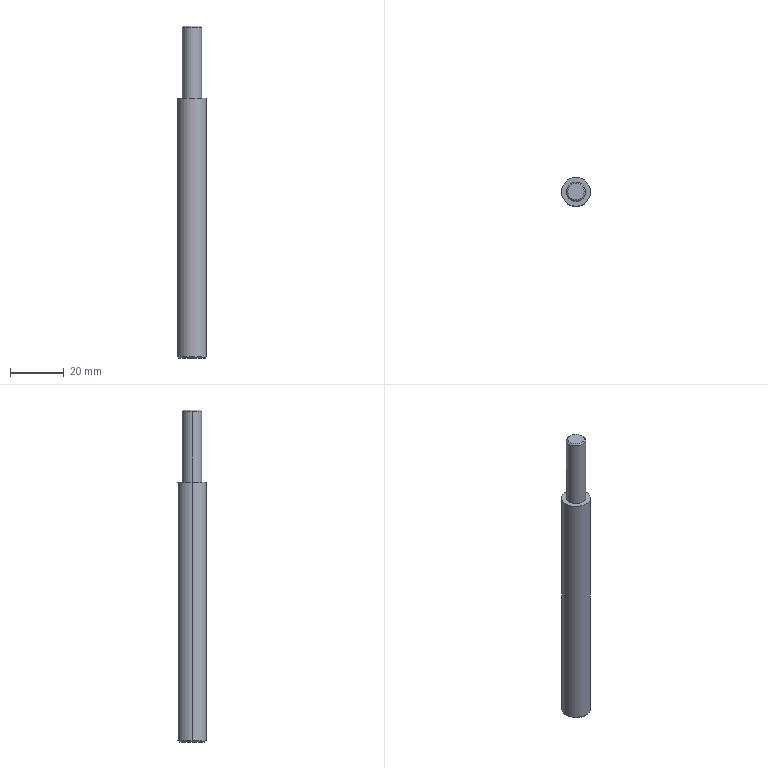Part | SolidWorks | features Chamfer 1, Extrusion 1, ICE 1 | 1 solid | 11 faces | box 10.8 x 10.8 x 124 mm | volume 9977 mm3 | cone 4 | cylinder 4 | plane 3 | commonest cylinder face diameters 7.2 x2 10.8 x2
STEP:
#1=CARTESIAN_POINT('',(3.06,0.,124.));
#2=VERTEX_POINT('',#1);
#3=CARTESIAN_POINT('',(-3.06,0.,124.));
#4=VERTEX_POINT('',#3);
#5=CARTESIAN_POINT('',(0.,0.,124.));
#6=DIRECTION('',(0.,0.,1.));
#7=DIRECTION('',(1.,0.,0.));
#8=AXIS2_PLACEMENT_3D('',#5,#6,#7);
#9=CIRCLE('',#8,3.06);
#10=EDGE_CURVE('',#2,#4,#9,.T.);
#11=ORIENTED_EDGE('',*,*,#10,.F.);
#12=CARTESIAN_POINT('',(3.6,0.,123.46));
#13=VERTEX_POINT('',#12);
#14=CARTESIAN_POINT('',(3.06,0.,124.));
#15=DIRECTION('',(0.7071,0.,-0.7071));
#16=VECTOR('',#15,1000.);
#17=LINE('',#14,#16);
#18=EDGE_CURVE('',#2,#13,#17,.T.);
#19=ORIENTED_EDGE('',*,*,#18,.T.);
#20=CARTESIAN_POINT('',(-3.6,0.,123.46));
#21=VERTEX_POINT('',#20);
#22=CARTESIAN_POINT('',(0.,0.,123.46));
#23=DIRECTION('',(0.,0.,-1.));
#24=DIRECTION('',(1.,0.,0.));
#25=AXIS2_PLACEMENT_3D('',#22,#23,#24);
#26=CIRCLE('',#25,3.6);
#27=EDGE_CURVE('',#21,#13,#26,.T.);
#28=ORIENTED_EDGE('',*,*,#27,.F.);
#29=CARTESIAN_POINT('',(-3.06,0.,124.));
#30=DIRECTION('',(-0.7071,0.,-0.7071));
#31=VECTOR('',#30,1000.);
#32=LINE('',#29,#31);
#33=EDGE_CURVE('',#4,#21,#32,.T.);
#34=ORIENTED_EDGE('',*,*,#33,.F.);
#35=EDGE_LOOP('',(#11,#19,#28,#34));
#36=FACE_OUTER_BOUND('',#35,.T.);
#37=CARTESIAN_POINT('',(0.,0.,124.));
#38=DIRECTION('',(0.,0.,-1.));
#39=DIRECTION('',(-1.,0.,0.));
#40=AXIS2_PLACEMENT_3D('',#37,#38,#39);
#41=CONICAL_SURFACE('',#40,3.06,0.7854);
#42=ADVANCED_FACE('',(#36),#41,.T.);
#43=CARTESIAN_POINT('',(-4.86,0.,0.));
#44=VERTEX_POINT('',#43);
#45=CARTESIAN_POINT('',(4.86,0.,0.));
#46=VERTEX_POINT('',#45);
#47=CARTESIAN_POINT('',(0.,0.,0.));
#48=DIRECTION('',(0.,0.,-1.));
#49=DIRECTION('',(1.,0.,0.));
#50=AXIS2_PLACEMENT_3D('',#47,#48,#49);
#51=CIRCLE('',#50,4.86);
#52=EDGE_CURVE('',#44,#46,#51,.T.);
#53=ORIENTED_EDGE('',*,*,#52,.F.);
#54=CARTESIAN_POINT('',(-5.4,0.,0.54));
#55=VERTEX_POINT('',#54);
#56=CARTESIAN_POINT('',(-5.4,0.,0.54));
#57=DIRECTION('',(-0.7071,0.,0.7071));
#58=VECTOR('',#57,1000.);
#59=LINE('',#56,#58);
#60=EDGE_CURVE('',#44,#55,#59,.T.);
#61=ORIENTED_EDGE('',*,*,#60,.T.);
#62=CARTESIAN_POINT('',(5.4,0.,0.54));
#63=VERTEX_POINT('',#62);
#64=CARTESIAN_POINT('',(0.,0.,0.54));
#65=DIRECTION('',(0.,0.,1.));
#66=DIRECTION('',(1.,0.,0.));
#67=AXIS2_PLACEMENT_3D('',#64,#65,#66);
#68=CIRCLE('',#67,5.4);
#69=EDGE_CURVE('',#63,#55,#68,.T.);
#70=ORIENTED_EDGE('',*,*,#69,.F.);
#71=CARTESIAN_POINT('',(5.4,0.,0.54));
#72=DIRECTION('',(0.7071,0.,0.7071));
#73=VECTOR('',#72,1000.);
#74=LINE('',#71,#73);
#75=EDGE_CURVE('',#46,#63,#74,.T.);
#76=ORIENTED_EDGE('',*,*,#75,.F.);
#77=EDGE_LOOP('',(#53,#61,#70,#76));
#78=FACE_OUTER_BOUND('',#77,.T.);
#79=CARTESIAN_POINT('',(0.,0.,0.54));
#80=DIRECTION('',(0.,0.,1.));
#81=DIRECTION('',(1.,0.,0.));
#82=AXIS2_PLACEMENT_3D('',#79,#80,#81);
#83=CONICAL_SURFACE('',#82,5.4,0.7854);
#84=ADVANCED_FACE('',(#78),#83,.T.);
#85=CARTESIAN_POINT('',(3.6,0.,97.));
#86=VERTEX_POINT('',#85);
#87=CARTESIAN_POINT('',(-3.6,0.,97.));
#88=VERTEX_POINT('',#87);
#89=CARTESIAN_POINT('',(0.,0.,97.));
#90=DIRECTION('',(0.,0.,1.));
#91=DIRECTION('',(1.,0.,0.));
#92=AXIS2_PLACEMENT_3D('',#89,#90,#91);
#93=CIRCLE('',#92,3.6);
#94=EDGE_CURVE('',#86,#88,#93,.T.);
#95=ORIENTED_EDGE('',*,*,#94,.T.);
#96=CARTESIAN_POINT('',(-3.6,0.,97.));
#97=DIRECTION('',(0.,0.,1.));
#98=VECTOR('',#97,1000.);
#99=LINE('',#96,#98);
#100=EDGE_CURVE('',#88,#21,#99,.T.);
#101=ORIENTED_EDGE('',*,*,#100,.T.);
#102=ORIENTED_EDGE('',*,*,#27,.T.);
#103=CARTESIAN_POINT('',(3.6,0.,97.));
#104=DIRECTION('',(0.,0.,1.));
#105=VECTOR('',#104,1000.);
#106=LINE('',#103,#105);
#107=EDGE_CURVE('',#86,#13,#106,.T.);
#108=ORIENTED_EDGE('',*,*,#107,.F.);
#109=EDGE_LOOP('',(#95,#101,#102,#108));
#110=FACE_OUTER_BOUND('',#109,.T.);
#111=CARTESIAN_POINT('',(0.,0.,97.));
#112=DIRECTION('',(0.,0.,1.));
#113=DIRECTION('',(1.,0.,0.));
#114=AXIS2_PLACEMENT_3D('',#111,#112,#113);
#115=CYLINDRICAL_SURFACE('',#114,3.6);
#116=ADVANCED_FACE('',(#110),#115,.T.);
#117=CARTESIAN_POINT('',(5.4,0.,97.));
#118=VERTEX_POINT('',#117);
#119=CARTESIAN_POINT('',(-5.4,0.,97.));
#120=VERTEX_POINT('',#119);
#121=CARTESIAN_POINT('',(0.,0.,97.));
#122=DIRECTION('',(0.,0.,1.));
#123=DIRECTION('',(1.,0.,0.));
#124=AXIS2_PLACEMENT_3D('',#121,#122,#123);
#125=CIRCLE('',#124,5.4);
#126=EDGE_CURVE('',#118,#120,#125,.T.);
#127=ORIENTED_EDGE('',*,*,#126,.F.);
#128=CARTESIAN_POINT('',(5.4,0.,124.));
#129=DIRECTION('',(0.,0.,-1.));
#130=VECTOR('',#129,1000.);
#131=LINE('',#128,#130);
#132=EDGE_CURVE('',#118,#63,#131,.T.);
#133=ORIENTED_EDGE('',*,*,#132,.T.);
#134=ORIENTED_EDGE('',*,*,#69,.T.);
#135=CARTESIAN_POINT('',(-5.4,0.,124.));
#136=DIRECTION('',(0.,0.,-1.));
#137=VECTOR('',#136,1000.);
#138=LINE('',#135,#137);
#139=EDGE_CURVE('',#120,#55,#138,.T.);
#140=ORIENTED_EDGE('',*,*,#139,.F.);
#141=EDGE_LOOP('',(#127,#133,#134,#140));
#142=FACE_OUTER_BOUND('',#141,.T.);
#143=CARTESIAN_POINT('',(0.,0.,124.));
#144=DIRECTION('',(0.,0.,-1.));
#145=DIRECTION('',(-1.,0.,0.));
#146=AXIS2_PLACEMENT_3D('',#143,#144,#145);
#147=CYLINDRICAL_SURFACE('',#146,5.4);
#148=ADVANCED_FACE('',(#142),#147,.T.);
#149=ORIENTED_EDGE('',*,*,#132,.F.);
#150=CARTESIAN_POINT('',(0.,0.,97.));
#151=DIRECTION('',(0.,0.,1.));
#152=DIRECTION('',(1.,0.,0.));
#153=AXIS2_PLACEMENT_3D('',#150,#151,#152);
#154=CIRCLE('',#153,5.4);
#155=EDGE_CURVE('',#120,#118,#154,.T.);
#156=ORIENTED_EDGE('',*,*,#155,.F.);
#157=ORIENTED_EDGE('',*,*,#139,.T.);
#158=CARTESIAN_POINT('',(0.,0.,0.54));
#159=DIRECTION('',(0.,0.,1.));
#160=DIRECTION('',(1.,0.,0.));
#161=AXIS2_PLACEMENT_3D('',#158,#159,#160);
#162=CIRCLE('',#161,5.4);
#163=EDGE_CURVE('',#55,#63,#162,.T.);
#164=ORIENTED_EDGE('',*,*,#163,.T.);
#165=EDGE_LOOP('',(#149,#156,#157,#164));
#166=FACE_OUTER_BOUND('',#165,.T.);
#167=CARTESIAN_POINT('',(0.,0.,124.));
#168=DIRECTION('',(0.,0.,-1.));
#169=DIRECTION('',(-1.,0.,0.));
#170=AXIS2_PLACEMENT_3D('',#167,#168,#169);
#171=CYLINDRICAL_SURFACE('',#170,5.4);
#172=ADVANCED_FACE('',(#166),#171,.T.);
#173=CARTESIAN_POINT('',(0.,0.,0.));
#174=DIRECTION('',(0.,0.,-1.));
#175=DIRECTION('',(1.,0.,0.));
#176=AXIS2_PLACEMENT_3D('',#173,#174,#175);
#177=CIRCLE('',#176,4.86);
#178=EDGE_CURVE('',#46,#44,#177,.T.);
#179=ORIENTED_EDGE('',*,*,#178,.T.);
#180=ORIENTED_EDGE('',*,*,#52,.T.);
#181=EDGE_LOOP('',(#179,#180));
#182=FACE_OUTER_BOUND('',#181,.T.);
#183=CARTESIAN_POINT('',(0.,0.,0.));
#184=DIRECTION('',(0.,0.,1.));
#185=DIRECTION('',(1.,0.,0.));
#186=AXIS2_PLACEMENT_3D('',#183,#184,#185);
#187=PLANE('',#186);
#188=ADVANCED_FACE('',(#182),#187,.F.);
#189=ORIENTED_EDGE('',*,*,#94,.F.);
#190=CARTESIAN_POINT('',(0.,0.,97.));
#191=DIRECTION('',(0.,0.,1.));
#192=DIRECTION('',(1.,0.,0.));
#193=AXIS2_PLACEMENT_3D('',#190,#191,#192);
#194=CIRCLE('',#193,3.6);
#195=EDGE_CURVE('',#88,#86,#194,.T.);
#196=ORIENTED_EDGE('',*,*,#195,.F.);
#197=EDGE_LOOP('',(#189,#196));
#198=FACE_BOUND('',#197,.T.);
#199=ORIENTED_EDGE('',*,*,#155,.T.);
#200=ORIENTED_EDGE('',*,*,#126,.T.);
#201=EDGE_LOOP('',(#199,#200));
#202=FACE_OUTER_BOUND('',#201,.T.);
#203=CARTESIAN_POINT('',(0.,0.,97.));
#204=DIRECTION('',(0.,0.,1.));
#205=DIRECTION('',(1.,0.,0.));
#206=AXIS2_PLACEMENT_3D('',#203,#204,#205);
#207=PLANE('',#206);
#208=ADVANCED_FACE('',(#198,#202),#207,.T.);
#209=ORIENTED_EDGE('',*,*,#100,.F.);
#210=ORIENTED_EDGE('',*,*,#195,.T.);
#211=ORIENTED_EDGE('',*,*,#107,.T.);
#212=CARTESIAN_POINT('',(0.,0.,123.46));
#213=DIRECTION('',(0.,0.,-1.));
#214=DIRECTION('',(1.,0.,0.));
#215=AXIS2_PLACEMENT_3D('',#212,#213,#214);
#216=CIRCLE('',#215,3.6);
#217=EDGE_CURVE('',#13,#21,#216,.T.);
#218=ORIENTED_EDGE('',*,*,#217,.T.);
#219=EDGE_LOOP('',(#209,#210,#211,#218));
#220=FACE_OUTER_BOUND('',#219,.T.);
#221=CARTESIAN_POINT('',(0.,0.,97.));
#222=DIRECTION('',(0.,0.,1.));
#223=DIRECTION('',(1.,0.,0.));
#224=AXIS2_PLACEMENT_3D('',#221,#222,#223);
#225=CYLINDRICAL_SURFACE('',#224,3.6);
#226=ADVANCED_FACE('',(#220),#225,.T.);
#227=CARTESIAN_POINT('',(0.,0.,124.));
#228=DIRECTION('',(0.,0.,1.));
#229=DIRECTION('',(1.,0.,0.));
#230=AXIS2_PLACEMENT_3D('',#227,#228,#229);
#231=CIRCLE('',#230,3.06);
#232=EDGE_CURVE('',#4,#2,#231,.T.);
#233=ORIENTED_EDGE('',*,*,#232,.T.);
#234=ORIENTED_EDGE('',*,*,#10,.T.);
#235=EDGE_LOOP('',(#233,#234));
#236=FACE_OUTER_BOUND('',#235,.T.);
#237=CARTESIAN_POINT('',(0.,0.,124.));
#238=DIRECTION('',(0.,0.,1.));
#239=DIRECTION('',(1.,0.,0.));
#240=AXIS2_PLACEMENT_3D('',#237,#238,#239);
#241=PLANE('',#240);
#242=ADVANCED_FACE('',(#236),#241,.T.);
#243=ORIENTED_EDGE('',*,*,#60,.F.);
#244=ORIENTED_EDGE('',*,*,#178,.F.);
#245=ORIENTED_EDGE('',*,*,#75,.T.);
#246=ORIENTED_EDGE('',*,*,#163,.F.);
#247=EDGE_LOOP('',(#243,#244,#245,#246));
#248=FACE_OUTER_BOUND('',#247,.T.);
#249=CARTESIAN_POINT('',(0.,0.,0.54));
#250=DIRECTION('',(0.,0.,1.));
#251=DIRECTION('',(1.,0.,0.));
#252=AXIS2_PLACEMENT_3D('',#249,#250,#251);
#253=CONICAL_SURFACE('',#252,5.4,0.7854);
#254=ADVANCED_FACE('',(#248),#253,.T.);
#255=ORIENTED_EDGE('',*,*,#18,.F.);
#256=ORIENTED_EDGE('',*,*,#232,.F.);
#257=ORIENTED_EDGE('',*,*,#33,.T.);
#258=ORIENTED_EDGE('',*,*,#217,.F.);
#259=EDGE_LOOP('',(#255,#256,#257,#258));
#260=FACE_OUTER_BOUND('',#259,.T.);
#261=CARTESIAN_POINT('',(0.,0.,124.));
#262=DIRECTION('',(0.,0.,-1.));
#263=DIRECTION('',(-1.,0.,0.));
#264=AXIS2_PLACEMENT_3D('',#261,#262,#263);
#265=CONICAL_SURFACE('',#264,3.06,0.7854);
#266=ADVANCED_FACE('',(#260),#265,.T.);
#267=CLOSED_SHELL('',(#42,#84,#116,#148,#172,#188,#208,#226,#242,#254,#266));
#268=MANIFOLD_SOLID_BREP('',#267);
#269=CARTESIAN_POINT('',(0.,0.,0.));
#270=DIRECTION('',(0.,0.,1.));
#271=DIRECTION('',(1.,0.,0.));
#272=AXIS2_PLACEMENT_3D('',#269,#270,#271);
#273=(LENGTH_UNIT()NAMED_UNIT(*)SI_UNIT(.MILLI.,.METRE.));
#274=UNCERTAINTY_MEASURE_WITH_UNIT(LENGTH_MEASURE(0.00001),#273,'','');
#275=(NAMED_UNIT(*)PLANE_ANGLE_UNIT()SI_UNIT($,.RADIAN.));
#276=(NAMED_UNIT(*)SI_UNIT($,.STERADIAN.)SOLID_ANGLE_UNIT());
#277=(GEOMETRIC_REPRESENTATION_CONTEXT(3)GLOBAL_UNCERTAINTY_ASSIGNED_CONTEXT((#274))GLOBAL_UNIT_ASSIGNED_CONTEXT((#273,#275,#276))REPRESENTATION_CONTEXT('',''));
#278=ADVANCED_BREP_SHAPE_REPRESENTATION('',(#268,#272),#277);